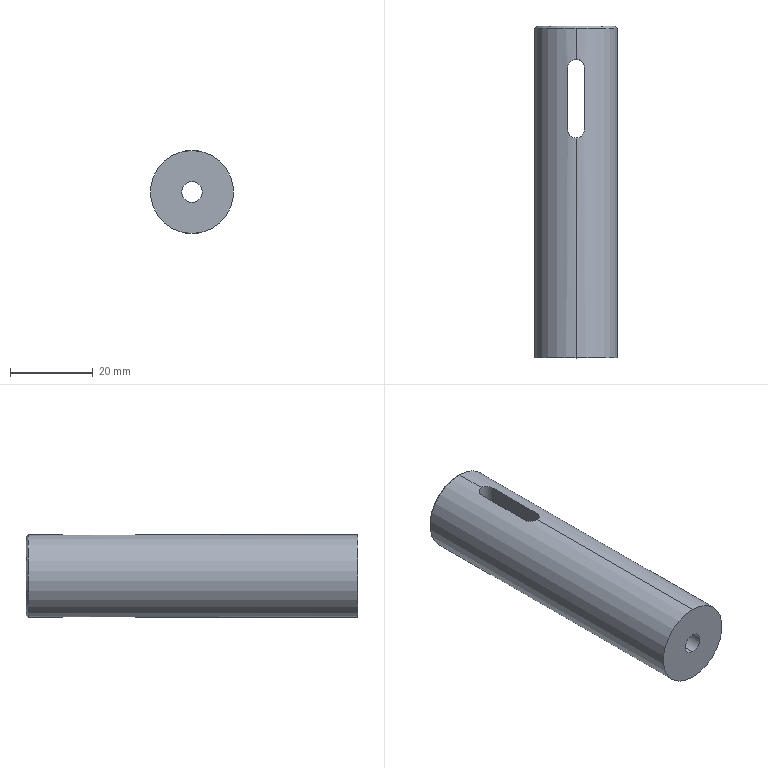Part | STEP file | PN_0054 | 1 solid | 19 faces | box 20 x 80 x 20 mm | volume 15788 mm3 | cylinder 10 | plane 7 | cone 2 | commonest cylinder face diameters 4 x4 5 x2 12.5 x2 20 x2